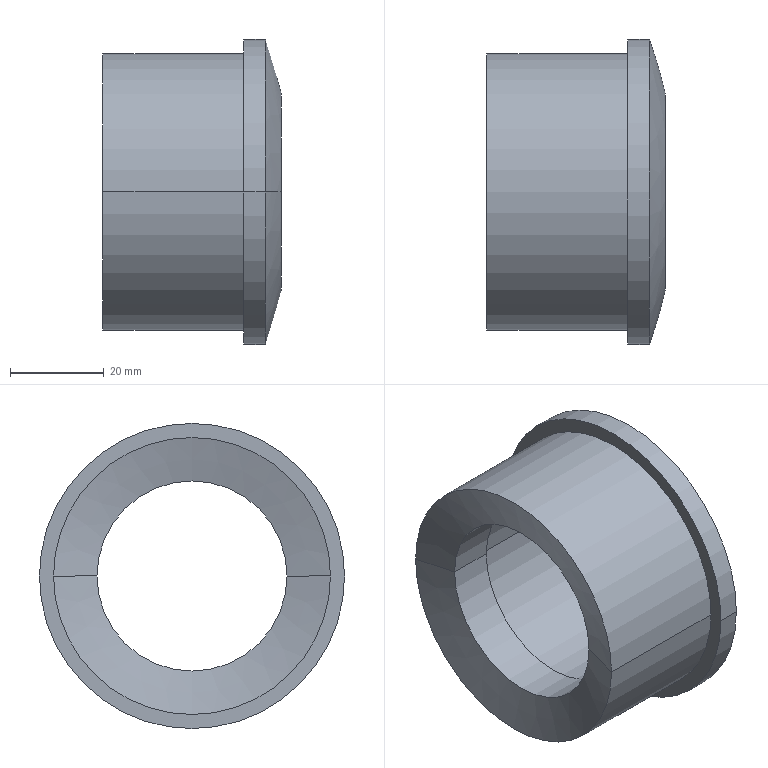Part | SolidWorks | features ICE 3, Revolution 1 | 1 solid | 14 faces | box 38 x 65 x 65 mm | volume 52156 mm3 | cylinder 8 | cone 2 | sphere 2 | plane 2 | commonest cylinder face diameters 40.5 x2 42 x2 59 x2 65 x2
STEP:
#1=CARTESIAN_POINT('',(38.,21.,0.));
#2=VERTEX_POINT('',#1);
#3=CARTESIAN_POINT('',(38.,-21.,0.));
#4=VERTEX_POINT('',#3);
#5=CARTESIAN_POINT('',(38.,0.,0.));
#6=DIRECTION('',(-1.,0.,0.));
#7=DIRECTION('',(0.,-1.,0.));
#8=AXIS2_PLACEMENT_3D('',#5,#6,#7);
#9=CIRCLE('',#8,21.);
#10=EDGE_CURVE('',#2,#4,#9,.T.);
#11=ORIENTED_EDGE('',*,*,#10,.F.);
#12=CARTESIAN_POINT('',(12.,21.,0.));
#13=VERTEX_POINT('',#12);
#14=CARTESIAN_POINT('',(38.,21.,0.));
#15=DIRECTION('',(-1.,0.,0.));
#16=VECTOR('',#15,1000.);
#17=LINE('',#14,#16);
#18=EDGE_CURVE('',#2,#13,#17,.T.);
#19=ORIENTED_EDGE('',*,*,#18,.T.);
#20=CARTESIAN_POINT('',(12.,-21.,0.));
#21=VERTEX_POINT('',#20);
#22=CARTESIAN_POINT('',(12.,0.,0.));
#23=DIRECTION('',(-1.,0.,0.));
#24=DIRECTION('',(0.,-1.,0.));
#25=AXIS2_PLACEMENT_3D('',#22,#23,#24);
#26=CIRCLE('',#25,21.);
#27=EDGE_CURVE('',#13,#21,#26,.T.);
#28=ORIENTED_EDGE('',*,*,#27,.T.);
#29=CARTESIAN_POINT('',(38.,-21.,0.));
#30=DIRECTION('',(-1.,0.,0.));
#31=VECTOR('',#30,1000.);
#32=LINE('',#29,#31);
#33=EDGE_CURVE('',#4,#21,#32,.T.);
#34=ORIENTED_EDGE('',*,*,#33,.F.);
#35=EDGE_LOOP('',(#11,#19,#28,#34));
#36=FACE_OUTER_BOUND('',#35,.T.);
#37=CARTESIAN_POINT('',(38.,0.,0.));
#38=DIRECTION('',(-1.,0.,0.));
#39=DIRECTION('',(0.,-1.,0.));
#40=AXIS2_PLACEMENT_3D('',#37,#38,#39);
#41=CYLINDRICAL_SURFACE('',#40,21.);
#42=ADVANCED_FACE('',(#36),#41,.F.);
#43=CARTESIAN_POINT('',(12.,20.25,0.));
#44=VERTEX_POINT('',#43);
#45=CARTESIAN_POINT('',(12.,-20.25,0.));
#46=VERTEX_POINT('',#45);
#47=CARTESIAN_POINT('',(12.,0.,0.));
#48=DIRECTION('',(-1.,0.,0.));
#49=DIRECTION('',(0.,-1.,0.));
#50=AXIS2_PLACEMENT_3D('',#47,#48,#49);
#51=CIRCLE('',#50,20.25);
#52=EDGE_CURVE('',#44,#46,#51,.T.);
#53=ORIENTED_EDGE('',*,*,#52,.F.);
#54=CARTESIAN_POINT('',(2.479,20.25,0.));
#55=VERTEX_POINT('',#54);
#56=CARTESIAN_POINT('',(12.,20.25,0.));
#57=DIRECTION('',(-1.,0.,0.));
#58=VECTOR('',#57,1000.);
#59=LINE('',#56,#58);
#60=EDGE_CURVE('',#44,#55,#59,.T.);
#61=ORIENTED_EDGE('',*,*,#60,.T.);
#62=CARTESIAN_POINT('',(2.479,-20.25,0.));
#63=VERTEX_POINT('',#62);
#64=CARTESIAN_POINT('',(2.479,0.,0.));
#65=DIRECTION('',(-1.,0.,0.));
#66=DIRECTION('',(0.,-1.,0.));
#67=AXIS2_PLACEMENT_3D('',#64,#65,#66);
#68=CIRCLE('',#67,20.25);
#69=EDGE_CURVE('',#55,#63,#68,.T.);
#70=ORIENTED_EDGE('',*,*,#69,.T.);
#71=CARTESIAN_POINT('',(12.,-20.25,0.));
#72=DIRECTION('',(-1.,0.,0.));
#73=VECTOR('',#72,1000.);
#74=LINE('',#71,#73);
#75=EDGE_CURVE('',#46,#63,#74,.T.);
#76=ORIENTED_EDGE('',*,*,#75,.F.);
#77=EDGE_LOOP('',(#53,#61,#70,#76));
#78=FACE_OUTER_BOUND('',#77,.T.);
#79=CARTESIAN_POINT('',(12.,0.,0.));
#80=DIRECTION('',(-1.,0.,0.));
#81=DIRECTION('',(0.,-1.,0.));
#82=AXIS2_PLACEMENT_3D('',#79,#80,#81);
#83=CYLINDRICAL_SURFACE('',#82,20.25);
#84=ADVANCED_FACE('',(#78),#83,.F.);
#85=ORIENTED_EDGE('',*,*,#69,.F.);
#86=CARTESIAN_POINT('',(0.,29.5,0.));
#87=VERTEX_POINT('',#86);
#88=CARTESIAN_POINT('',(0.,29.5,0.));
#89=DIRECTION('',(-0.2588,0.9659,0.));
#90=VECTOR('',#89,1000.);
#91=LINE('',#88,#90);
#92=EDGE_CURVE('',#55,#87,#91,.T.);
#93=ORIENTED_EDGE('',*,*,#92,.T.);
#94=CARTESIAN_POINT('',(0.,-29.5,0.));
#95=VERTEX_POINT('',#94);
#96=CARTESIAN_POINT('',(0.,0.,0.));
#97=DIRECTION('',(-1.,0.,0.));
#98=DIRECTION('',(0.,-1.,0.));
#99=AXIS2_PLACEMENT_3D('',#96,#97,#98);
#100=CIRCLE('',#99,29.5);
#101=EDGE_CURVE('',#87,#95,#100,.T.);
#102=ORIENTED_EDGE('',*,*,#101,.T.);
#103=CARTESIAN_POINT('',(0.,-29.5,0.));
#104=DIRECTION('',(-0.2588,-0.9659,0.));
#105=VECTOR('',#104,1000.);
#106=LINE('',#103,#105);
#107=EDGE_CURVE('',#63,#95,#106,.T.);
#108=ORIENTED_EDGE('',*,*,#107,.F.);
#109=EDGE_LOOP('',(#85,#93,#102,#108));
#110=FACE_OUTER_BOUND('',#109,.T.);
#111=CARTESIAN_POINT('',(0.,0.,0.));
#112=DIRECTION('',(-1.,0.,0.));
#113=DIRECTION('',(0.,-1.,0.));
#114=AXIS2_PLACEMENT_3D('',#111,#112,#113);
#115=CONICAL_SURFACE('',#114,29.5,1.309);
#116=ADVANCED_FACE('',(#110),#115,.F.);
#117=CARTESIAN_POINT('',(34.618,32.5,0.));
#118=VERTEX_POINT('',#117);
#119=CARTESIAN_POINT('',(34.618,-32.5,0.));
#120=VERTEX_POINT('',#119);
#121=CARTESIAN_POINT('',(34.618,0.,0.));
#122=DIRECTION('',(1.,0.,0.));
#123=DIRECTION('',(0.,1.,0.));
#124=AXIS2_PLACEMENT_3D('',#121,#122,#123);
#125=CIRCLE('',#124,32.5);
#126=EDGE_CURVE('',#118,#120,#125,.T.);
#127=ORIENTED_EDGE('',*,*,#126,.T.);
#128=CARTESIAN_POINT('',(-54.65,0.,0.));
#129=DIRECTION('',(0.,0.,1.));
#130=DIRECTION('',(0.,-1.,0.));
#131=AXIS2_PLACEMENT_3D('',#128,#129,#130);
#132=CIRCLE('',#131,95.);
#133=EDGE_CURVE('',#120,#4,#132,.T.);
#134=ORIENTED_EDGE('',*,*,#133,.T.);
#135=CARTESIAN_POINT('',(38.,0.,0.));
#136=DIRECTION('',(-1.,0.,0.));
#137=DIRECTION('',(0.,-1.,0.));
#138=AXIS2_PLACEMENT_3D('',#135,#136,#137);
#139=CIRCLE('',#138,21.);
#140=EDGE_CURVE('',#4,#2,#139,.T.);
#141=ORIENTED_EDGE('',*,*,#140,.T.);
#142=CARTESIAN_POINT('',(-54.65,0.,0.));
#143=DIRECTION('',(0.,0.,-1.));
#144=DIRECTION('',(-1.,0.,0.));
#145=AXIS2_PLACEMENT_3D('',#142,#143,#144);
#146=CIRCLE('',#145,95.);
#147=EDGE_CURVE('',#118,#2,#146,.T.);
#148=ORIENTED_EDGE('',*,*,#147,.F.);
#149=EDGE_LOOP('',(#127,#134,#141,#148));
#150=FACE_OUTER_BOUND('',#149,.T.);
#151=CARTESIAN_POINT('',(-54.65,0.,0.));
#152=DIRECTION('',(0.,0.,1.));
#153=DIRECTION('',(0.,1.,0.));
#154=AXIS2_PLACEMENT_3D('',#151,#152,#153);
#155=SPHERICAL_SURFACE('',#154,95.);
#156=ADVANCED_FACE('',(#150),#155,.T.);
#157=CARTESIAN_POINT('',(30.,32.5,0.));
#158=VERTEX_POINT('',#157);
#159=CARTESIAN_POINT('',(30.,-32.5,0.));
#160=VERTEX_POINT('',#159);
#161=CARTESIAN_POINT('',(30.,0.,0.));
#162=DIRECTION('',(1.,0.,0.));
#163=DIRECTION('',(0.,1.,0.));
#164=AXIS2_PLACEMENT_3D('',#161,#162,#163);
#165=CIRCLE('',#164,32.5);
#166=EDGE_CURVE('',#158,#160,#165,.T.);
#167=ORIENTED_EDGE('',*,*,#166,.T.);
#168=CARTESIAN_POINT('',(38.,-32.5,0.));
#169=DIRECTION('',(1.,0.,0.));
#170=VECTOR('',#169,1000.);
#171=LINE('',#168,#170);
#172=EDGE_CURVE('',#160,#120,#171,.T.);
#173=ORIENTED_EDGE('',*,*,#172,.T.);
#174=ORIENTED_EDGE('',*,*,#126,.F.);
#175=CARTESIAN_POINT('',(38.,32.5,0.));
#176=DIRECTION('',(1.,0.,0.));
#177=VECTOR('',#176,1000.);
#178=LINE('',#175,#177);
#179=EDGE_CURVE('',#158,#118,#178,.T.);
#180=ORIENTED_EDGE('',*,*,#179,.F.);
#181=EDGE_LOOP('',(#167,#173,#174,#180));
#182=FACE_OUTER_BOUND('',#181,.T.);
#183=CARTESIAN_POINT('',(38.,0.,0.));
#184=DIRECTION('',(1.,0.,0.));
#185=DIRECTION('',(0.,1.,0.));
#186=AXIS2_PLACEMENT_3D('',#183,#184,#185);
#187=CYLINDRICAL_SURFACE('',#186,32.5);
#188=ADVANCED_FACE('',(#182),#187,.T.);
#189=CARTESIAN_POINT('',(0.,0.,0.));
#190=DIRECTION('',(-1.,0.,0.));
#191=DIRECTION('',(0.,-1.,0.));
#192=AXIS2_PLACEMENT_3D('',#189,#190,#191);
#193=CIRCLE('',#192,29.5);
#194=EDGE_CURVE('',#95,#87,#193,.T.);
#195=ORIENTED_EDGE('',*,*,#194,.F.);
#196=CARTESIAN_POINT('',(30.,-29.5,0.));
#197=VERTEX_POINT('',#196);
#198=CARTESIAN_POINT('',(38.,-29.5,0.));
#199=DIRECTION('',(1.,0.,0.));
#200=VECTOR('',#199,1000.);
#201=LINE('',#198,#200);
#202=EDGE_CURVE('',#95,#197,#201,.T.);
#203=ORIENTED_EDGE('',*,*,#202,.T.);
#204=CARTESIAN_POINT('',(30.,29.5,0.));
#205=VERTEX_POINT('',#204);
#206=CARTESIAN_POINT('',(30.,0.,0.));
#207=DIRECTION('',(1.,0.,0.));
#208=DIRECTION('',(0.,1.,0.));
#209=AXIS2_PLACEMENT_3D('',#206,#207,#208);
#210=CIRCLE('',#209,29.5);
#211=EDGE_CURVE('',#205,#197,#210,.T.);
#212=ORIENTED_EDGE('',*,*,#211,.F.);
#213=CARTESIAN_POINT('',(38.,29.5,0.));
#214=DIRECTION('',(1.,0.,0.));
#215=VECTOR('',#214,1000.);
#216=LINE('',#213,#215);
#217=EDGE_CURVE('',#87,#205,#216,.T.);
#218=ORIENTED_EDGE('',*,*,#217,.F.);
#219=EDGE_LOOP('',(#195,#203,#212,#218));
#220=FACE_OUTER_BOUND('',#219,.T.);
#221=CARTESIAN_POINT('',(38.,0.,0.));
#222=DIRECTION('',(1.,0.,0.));
#223=DIRECTION('',(0.,1.,0.));
#224=AXIS2_PLACEMENT_3D('',#221,#222,#223);
#225=CYLINDRICAL_SURFACE('',#224,29.5);
#226=ADVANCED_FACE('',(#220),#225,.T.);
#227=ORIENTED_EDGE('',*,*,#202,.F.);
#228=ORIENTED_EDGE('',*,*,#101,.F.);
#229=ORIENTED_EDGE('',*,*,#217,.T.);
#230=CARTESIAN_POINT('',(30.,0.,0.));
#231=DIRECTION('',(1.,0.,0.));
#232=DIRECTION('',(0.,1.,0.));
#233=AXIS2_PLACEMENT_3D('',#230,#231,#232);
#234=CIRCLE('',#233,29.5);
#235=EDGE_CURVE('',#197,#205,#234,.T.);
#236=ORIENTED_EDGE('',*,*,#235,.F.);
#237=EDGE_LOOP('',(#227,#228,#229,#236));
#238=FACE_OUTER_BOUND('',#237,.T.);
#239=CARTESIAN_POINT('',(38.,0.,0.));
#240=DIRECTION('',(1.,0.,0.));
#241=DIRECTION('',(0.,1.,0.));
#242=AXIS2_PLACEMENT_3D('',#239,#240,#241);
#243=CYLINDRICAL_SURFACE('',#242,29.5);
#244=ADVANCED_FACE('',(#238),#243,.T.);
#245=ORIENTED_EDGE('',*,*,#211,.T.);
#246=ORIENTED_EDGE('',*,*,#235,.T.);
#247=EDGE_LOOP('',(#245,#246));
#248=FACE_BOUND('',#247,.T.);
#249=ORIENTED_EDGE('',*,*,#166,.F.);
#250=CARTESIAN_POINT('',(30.,0.,0.));
#251=DIRECTION('',(1.,0.,0.));
#252=DIRECTION('',(0.,1.,0.));
#253=AXIS2_PLACEMENT_3D('',#250,#251,#252);
#254=CIRCLE('',#253,32.5);
#255=EDGE_CURVE('',#160,#158,#254,.T.);
#256=ORIENTED_EDGE('',*,*,#255,.F.);
#257=EDGE_LOOP('',(#249,#256));
#258=FACE_OUTER_BOUND('',#257,.T.);
#259=CARTESIAN_POINT('',(30.,29.5,0.));
#260=DIRECTION('',(-1.,0.,0.));
#261=DIRECTION('',(0.,-1.,0.));
#262=AXIS2_PLACEMENT_3D('',#259,#260,#261);
#263=PLANE('',#262);
#264=ADVANCED_FACE('',(#248,#258),#263,.T.);
#265=ORIENTED_EDGE('',*,*,#172,.F.);
#266=ORIENTED_EDGE('',*,*,#255,.T.);
#267=ORIENTED_EDGE('',*,*,#179,.T.);
#268=CARTESIAN_POINT('',(34.618,0.,0.));
#269=DIRECTION('',(1.,0.,0.));
#270=DIRECTION('',(0.,1.,0.));
#271=AXIS2_PLACEMENT_3D('',#268,#269,#270);
#272=CIRCLE('',#271,32.5);
#273=EDGE_CURVE('',#120,#118,#272,.T.);
#274=ORIENTED_EDGE('',*,*,#273,.F.);
#275=EDGE_LOOP('',(#265,#266,#267,#274));
#276=FACE_OUTER_BOUND('',#275,.T.);
#277=CARTESIAN_POINT('',(38.,0.,0.));
#278=DIRECTION('',(1.,0.,0.));
#279=DIRECTION('',(0.,1.,0.));
#280=AXIS2_PLACEMENT_3D('',#277,#278,#279);
#281=CYLINDRICAL_SURFACE('',#280,32.5);
#282=ADVANCED_FACE('',(#276),#281,.T.);
#283=ORIENTED_EDGE('',*,*,#133,.F.);
#284=ORIENTED_EDGE('',*,*,#273,.T.);
#285=ORIENTED_EDGE('',*,*,#147,.T.);
#286=ORIENTED_EDGE('',*,*,#10,.T.);
#287=EDGE_LOOP('',(#283,#284,#285,#286));
#288=FACE_OUTER_BOUND('',#287,.T.);
#289=CARTESIAN_POINT('',(-54.65,0.,0.));
#290=DIRECTION('',(0.,0.,1.));
#291=DIRECTION('',(0.,1.,0.));
#292=AXIS2_PLACEMENT_3D('',#289,#290,#291);
#293=SPHERICAL_SURFACE('',#292,95.);
#294=ADVANCED_FACE('',(#288),#293,.T.);
#295=ORIENTED_EDGE('',*,*,#92,.F.);
#296=CARTESIAN_POINT('',(2.479,0.,0.));
#297=DIRECTION('',(-1.,0.,0.));
#298=DIRECTION('',(0.,-1.,0.));
#299=AXIS2_PLACEMENT_3D('',#296,#297,#298);
#300=CIRCLE('',#299,20.25);
#301=EDGE_CURVE('',#63,#55,#300,.T.);
#302=ORIENTED_EDGE('',*,*,#301,.F.);
#303=ORIENTED_EDGE('',*,*,#107,.T.);
#304=ORIENTED_EDGE('',*,*,#194,.T.);
#305=EDGE_LOOP('',(#295,#302,#303,#304));
#306=FACE_OUTER_BOUND('',#305,.T.);
#307=CARTESIAN_POINT('',(0.,0.,0.));
#308=DIRECTION('',(-1.,0.,0.));
#309=DIRECTION('',(0.,-1.,0.));
#310=AXIS2_PLACEMENT_3D('',#307,#308,#309);
#311=CONICAL_SURFACE('',#310,29.5,1.309);
#312=ADVANCED_FACE('',(#306),#311,.F.);
#313=ORIENTED_EDGE('',*,*,#60,.F.);
#314=CARTESIAN_POINT('',(12.,0.,0.));
#315=DIRECTION('',(-1.,0.,0.));
#316=DIRECTION('',(0.,-1.,0.));
#317=AXIS2_PLACEMENT_3D('',#314,#315,#316);
#318=CIRCLE('',#317,20.25);
#319=EDGE_CURVE('',#46,#44,#318,.T.);
#320=ORIENTED_EDGE('',*,*,#319,.F.);
#321=ORIENTED_EDGE('',*,*,#75,.T.);
#322=ORIENTED_EDGE('',*,*,#301,.T.);
#323=EDGE_LOOP('',(#313,#320,#321,#322));
#324=FACE_OUTER_BOUND('',#323,.T.);
#325=CARTESIAN_POINT('',(12.,0.,0.));
#326=DIRECTION('',(-1.,0.,0.));
#327=DIRECTION('',(0.,-1.,0.));
#328=AXIS2_PLACEMENT_3D('',#325,#326,#327);
#329=CYLINDRICAL_SURFACE('',#328,20.25);
#330=ADVANCED_FACE('',(#324),#329,.F.);
#331=ORIENTED_EDGE('',*,*,#18,.F.);
#332=ORIENTED_EDGE('',*,*,#140,.F.);
#333=ORIENTED_EDGE('',*,*,#33,.T.);
#334=CARTESIAN_POINT('',(12.,0.,0.));
#335=DIRECTION('',(-1.,0.,0.));
#336=DIRECTION('',(0.,-1.,0.));
#337=AXIS2_PLACEMENT_3D('',#334,#335,#336);
#338=CIRCLE('',#337,21.);
#339=EDGE_CURVE('',#21,#13,#338,.T.);
#340=ORIENTED_EDGE('',*,*,#339,.T.);
#341=EDGE_LOOP('',(#331,#332,#333,#340));
#342=FACE_OUTER_BOUND('',#341,.T.);
#343=CARTESIAN_POINT('',(38.,0.,0.));
#344=DIRECTION('',(-1.,0.,0.));
#345=DIRECTION('',(0.,-1.,0.));
#346=AXIS2_PLACEMENT_3D('',#343,#344,#345);
#347=CYLINDRICAL_SURFACE('',#346,21.);
#348=ADVANCED_FACE('',(#342),#347,.F.);
#349=ORIENTED_EDGE('',*,*,#319,.T.);
#350=ORIENTED_EDGE('',*,*,#52,.T.);
#351=EDGE_LOOP('',(#349,#350));
#352=FACE_BOUND('',#351,.T.);
#353=ORIENTED_EDGE('',*,*,#339,.F.);
#354=ORIENTED_EDGE('',*,*,#27,.F.);
#355=EDGE_LOOP('',(#353,#354));
#356=FACE_OUTER_BOUND('',#355,.T.);
#357=CARTESIAN_POINT('',(12.,0.,0.));
#358=DIRECTION('',(-1.,0.,0.));
#359=DIRECTION('',(0.,-1.,0.));
#360=AXIS2_PLACEMENT_3D('',#357,#358,#359);
#361=PLANE('',#360);
#362=ADVANCED_FACE('',(#352,#356),#361,.F.);
#363=CLOSED_SHELL('',(#42,#84,#116,#156,#188,#226,#244,#264,#282,#294,#312,#330,#348,#362));
#364=MANIFOLD_SOLID_BREP('',#363);
#365=CARTESIAN_POINT('',(0.,0.,0.));
#366=DIRECTION('',(0.,0.,1.));
#367=DIRECTION('',(1.,0.,0.));
#368=AXIS2_PLACEMENT_3D('',#365,#366,#367);
#369=(LENGTH_UNIT()NAMED_UNIT(*)SI_UNIT(.MILLI.,.METRE.));
#370=UNCERTAINTY_MEASURE_WITH_UNIT(LENGTH_MEASURE(0.00001),#369,'','');
#371=(NAMED_UNIT(*)PLANE_ANGLE_UNIT()SI_UNIT($,.RADIAN.));
#372=(NAMED_UNIT(*)SI_UNIT($,.STERADIAN.)SOLID_ANGLE_UNIT());
#373=(GEOMETRIC_REPRESENTATION_CONTEXT(3)GLOBAL_UNCERTAINTY_ASSIGNED_CONTEXT((#370))GLOBAL_UNIT_ASSIGNED_CONTEXT((#369,#371,#372))REPRESENTATION_CONTEXT('',''));
#374=ADVANCED_BREP_SHAPE_REPRESENTATION('',(#364,#368),#373);